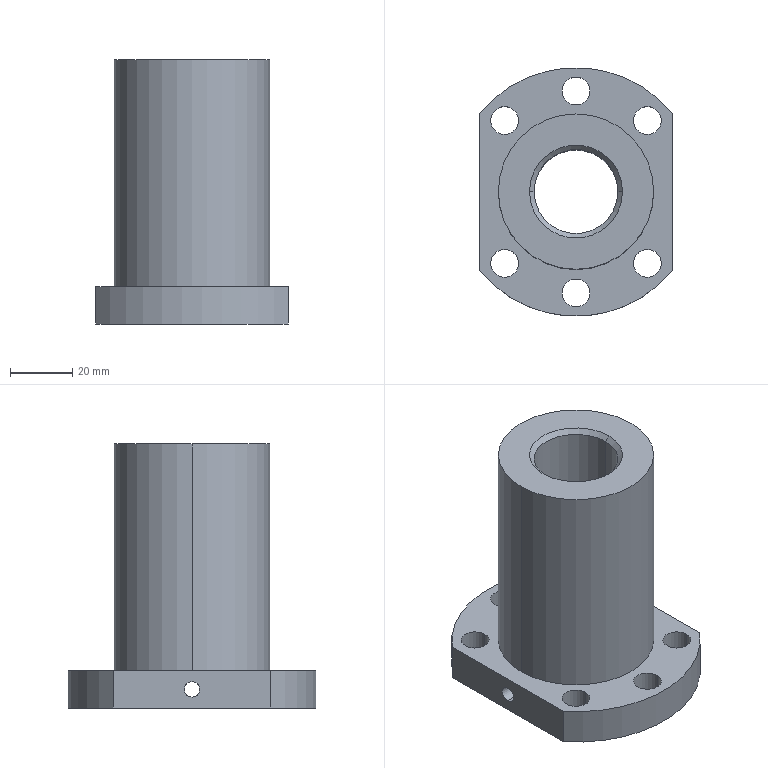Part | SolidWorks | features BaseBody 1 | 1 solid | 31 faces | box 62 x 80 x 85 mm | volume 142057 mm3 | cylinder 22 | plane 5 | cone 4 | commonest cylinder face diameters 9 x12 5 x4 27 x2 50 x2 80 x2
STEP:
#1=CARTESIAN_POINT('',(-25.,0.,85.));
#2=VERTEX_POINT('',#1);
#3=CARTESIAN_POINT('',(25.,0.,85.));
#4=VERTEX_POINT('',#3);
#5=CARTESIAN_POINT('',(0.,0.,85.));
#6=DIRECTION('',(0.,0.,-1.));
#7=DIRECTION('',(-1.,0.,0.));
#8=AXIS2_PLACEMENT_3D('',#5,#6,#7);
#9=CIRCLE('',#8,25.);
#10=EDGE_CURVE('',#2,#4,#9,.T.);
#11=ORIENTED_EDGE('',*,*,#10,.T.);
#12=CARTESIAN_POINT('',(25.,0.,12.));
#13=VERTEX_POINT('',#12);
#14=CARTESIAN_POINT('',(25.,0.,85.));
#15=DIRECTION('',(0.,0.,-1.));
#16=VECTOR('',#15,1000.);
#17=LINE('',#14,#16);
#18=EDGE_CURVE('',#4,#13,#17,.T.);
#19=ORIENTED_EDGE('',*,*,#18,.T.);
#20=CARTESIAN_POINT('',(-25.,0.,12.));
#21=VERTEX_POINT('',#20);
#22=CARTESIAN_POINT('',(0.,0.,12.));
#23=DIRECTION('',(0.,0.,1.));
#24=DIRECTION('',(-1.,0.,0.));
#25=AXIS2_PLACEMENT_3D('',#22,#23,#24);
#26=CIRCLE('',#25,25.);
#27=EDGE_CURVE('',#13,#21,#26,.T.);
#28=ORIENTED_EDGE('',*,*,#27,.T.);
#29=CARTESIAN_POINT('',(-25.,0.,85.));
#30=DIRECTION('',(0.,0.,-1.));
#31=VECTOR('',#30,1000.);
#32=LINE('',#29,#31);
#33=EDGE_CURVE('',#2,#21,#32,.T.);
#34=ORIENTED_EDGE('',*,*,#33,.F.);
#35=EDGE_LOOP('',(#11,#19,#28,#34));
#36=FACE_OUTER_BOUND('',#35,.T.);
#37=CARTESIAN_POINT('',(0.,0.,85.));
#38=DIRECTION('',(0.,0.,-1.));
#39=DIRECTION('',(-1.,0.,0.));
#40=AXIS2_PLACEMENT_3D('',#37,#38,#39);
#41=CYLINDRICAL_SURFACE('',#40,25.);
#42=ADVANCED_FACE('',(#36),#41,.T.);
#43=CARTESIAN_POINT('',(-18.481,-22.981,12.));
#44=VERTEX_POINT('',#43);
#45=CARTESIAN_POINT('',(-27.481,-22.981,12.));
#46=VERTEX_POINT('',#45);
#47=CARTESIAN_POINT('',(-22.981,-22.981,12.));
#48=DIRECTION('',(0.,0.,-1.));
#49=DIRECTION('',(-1.,0.,0.));
#50=AXIS2_PLACEMENT_3D('',#47,#48,#49);
#51=CIRCLE('',#50,4.5);
#52=EDGE_CURVE('',#44,#46,#51,.T.);
#53=ORIENTED_EDGE('',*,*,#52,.F.);
#54=CARTESIAN_POINT('',(-18.481,-22.981,0.));
#55=VERTEX_POINT('',#54);
#56=CARTESIAN_POINT('',(-18.481,-22.981,12.));
#57=DIRECTION('',(0.,0.,-1.));
#58=VECTOR('',#57,1000.);
#59=LINE('',#56,#58);
#60=EDGE_CURVE('',#44,#55,#59,.T.);
#61=ORIENTED_EDGE('',*,*,#60,.T.);
#62=CARTESIAN_POINT('',(-27.481,-22.981,0.));
#63=VERTEX_POINT('',#62);
#64=CARTESIAN_POINT('',(-22.981,-22.981,0.));
#65=DIRECTION('',(0.,0.,1.));
#66=DIRECTION('',(-1.,0.,0.));
#67=AXIS2_PLACEMENT_3D('',#64,#65,#66);
#68=CIRCLE('',#67,4.5);
#69=EDGE_CURVE('',#63,#55,#68,.T.);
#70=ORIENTED_EDGE('',*,*,#69,.F.);
#71=CARTESIAN_POINT('',(-27.481,-22.981,12.));
#72=DIRECTION('',(0.,0.,-1.));
#73=VECTOR('',#72,1000.);
#74=LINE('',#71,#73);
#75=EDGE_CURVE('',#46,#63,#74,.T.);
#76=ORIENTED_EDGE('',*,*,#75,.F.);
#77=EDGE_LOOP('',(#53,#61,#70,#76));
#78=FACE_OUTER_BOUND('',#77,.T.);
#79=CARTESIAN_POINT('',(-22.981,-22.981,12.));
#80=DIRECTION('',(0.,0.,-1.));
#81=DIRECTION('',(-1.,0.,0.));
#82=AXIS2_PLACEMENT_3D('',#79,#80,#81);
#83=CYLINDRICAL_SURFACE('',#82,4.5);
#84=ADVANCED_FACE('',(#78),#83,.F.);
#85=CARTESIAN_POINT('',(27.481,-22.981,12.));
#86=VERTEX_POINT('',#85);
#87=CARTESIAN_POINT('',(18.481,-22.981,12.));
#88=VERTEX_POINT('',#87);
#89=CARTESIAN_POINT('',(22.981,-22.981,12.));
#90=DIRECTION('',(0.,0.,-1.));
#91=DIRECTION('',(-1.,0.,0.));
#92=AXIS2_PLACEMENT_3D('',#89,#90,#91);
#93=CIRCLE('',#92,4.5);
#94=EDGE_CURVE('',#86,#88,#93,.T.);
#95=ORIENTED_EDGE('',*,*,#94,.F.);
#96=CARTESIAN_POINT('',(27.481,-22.981,0.));
#97=VERTEX_POINT('',#96);
#98=CARTESIAN_POINT('',(27.481,-22.981,12.));
#99=DIRECTION('',(0.,0.,-1.));
#100=VECTOR('',#99,1000.);
#101=LINE('',#98,#100);
#102=EDGE_CURVE('',#86,#97,#101,.T.);
#103=ORIENTED_EDGE('',*,*,#102,.T.);
#104=CARTESIAN_POINT('',(18.481,-22.981,0.));
#105=VERTEX_POINT('',#104);
#106=CARTESIAN_POINT('',(22.981,-22.981,0.));
#107=DIRECTION('',(0.,0.,1.));
#108=DIRECTION('',(-1.,0.,0.));
#109=AXIS2_PLACEMENT_3D('',#106,#107,#108);
#110=CIRCLE('',#109,4.5);
#111=EDGE_CURVE('',#105,#97,#110,.T.);
#112=ORIENTED_EDGE('',*,*,#111,.F.);
#113=CARTESIAN_POINT('',(18.481,-22.981,12.));
#114=DIRECTION('',(0.,0.,-1.));
#115=VECTOR('',#114,1000.);
#116=LINE('',#113,#115);
#117=EDGE_CURVE('',#88,#105,#116,.T.);
#118=ORIENTED_EDGE('',*,*,#117,.F.);
#119=EDGE_LOOP('',(#95,#103,#112,#118));
#120=FACE_OUTER_BOUND('',#119,.T.);
#121=CARTESIAN_POINT('',(22.981,-22.981,12.));
#122=DIRECTION('',(0.,0.,-1.));
#123=DIRECTION('',(-1.,0.,0.));
#124=AXIS2_PLACEMENT_3D('',#121,#122,#123);
#125=CYLINDRICAL_SURFACE('',#124,4.5);
#126=ADVANCED_FACE('',(#120),#125,.F.);
#127=CARTESIAN_POINT('',(27.481,22.981,12.));
#128=VERTEX_POINT('',#127);
#129=CARTESIAN_POINT('',(18.481,22.981,12.));
#130=VERTEX_POINT('',#129);
#131=CARTESIAN_POINT('',(22.981,22.981,12.));
#132=DIRECTION('',(0.,0.,-1.));
#133=DIRECTION('',(-1.,0.,0.));
#134=AXIS2_PLACEMENT_3D('',#131,#132,#133);
#135=CIRCLE('',#134,4.5);
#136=EDGE_CURVE('',#128,#130,#135,.T.);
#137=ORIENTED_EDGE('',*,*,#136,.F.);
#138=CARTESIAN_POINT('',(27.481,22.981,0.));
#139=VERTEX_POINT('',#138);
#140=CARTESIAN_POINT('',(27.481,22.981,12.));
#141=DIRECTION('',(0.,0.,-1.));
#142=VECTOR('',#141,1000.);
#143=LINE('',#140,#142);
#144=EDGE_CURVE('',#128,#139,#143,.T.);
#145=ORIENTED_EDGE('',*,*,#144,.T.);
#146=CARTESIAN_POINT('',(18.481,22.981,0.));
#147=VERTEX_POINT('',#146);
#148=CARTESIAN_POINT('',(22.981,22.981,0.));
#149=DIRECTION('',(0.,0.,1.));
#150=DIRECTION('',(-1.,0.,0.));
#151=AXIS2_PLACEMENT_3D('',#148,#149,#150);
#152=CIRCLE('',#151,4.5);
#153=EDGE_CURVE('',#147,#139,#152,.T.);
#154=ORIENTED_EDGE('',*,*,#153,.F.);
#155=CARTESIAN_POINT('',(18.481,22.981,12.));
#156=DIRECTION('',(0.,0.,-1.));
#157=VECTOR('',#156,1000.);
#158=LINE('',#155,#157);
#159=EDGE_CURVE('',#130,#147,#158,.T.);
#160=ORIENTED_EDGE('',*,*,#159,.F.);
#161=EDGE_LOOP('',(#137,#145,#154,#160));
#162=FACE_OUTER_BOUND('',#161,.T.);
#163=CARTESIAN_POINT('',(22.981,22.981,12.));
#164=DIRECTION('',(0.,0.,-1.));
#165=DIRECTION('',(-1.,0.,0.));
#166=AXIS2_PLACEMENT_3D('',#163,#164,#165);
#167=CYLINDRICAL_SURFACE('',#166,4.5);
#168=ADVANCED_FACE('',(#162),#167,.F.);
#169=CARTESIAN_POINT('',(4.5,32.5,12.));
#170=VERTEX_POINT('',#169);
#171=CARTESIAN_POINT('',(-4.5,32.5,12.));
#172=VERTEX_POINT('',#171);
#173=CARTESIAN_POINT('',(0.,32.5,12.));
#174=DIRECTION('',(0.,0.,-1.));
#175=DIRECTION('',(-1.,0.,0.));
#176=AXIS2_PLACEMENT_3D('',#173,#174,#175);
#177=CIRCLE('',#176,4.5);
#178=EDGE_CURVE('',#170,#172,#177,.T.);
#179=ORIENTED_EDGE('',*,*,#178,.F.);
#180=CARTESIAN_POINT('',(4.5,32.5,0.));
#181=VERTEX_POINT('',#180);
#182=CARTESIAN_POINT('',(4.5,32.5,12.));
#183=DIRECTION('',(0.,0.,-1.));
#184=VECTOR('',#183,1000.);
#185=LINE('',#182,#184);
#186=EDGE_CURVE('',#170,#181,#185,.T.);
#187=ORIENTED_EDGE('',*,*,#186,.T.);
#188=CARTESIAN_POINT('',(-4.5,32.5,0.));
#189=VERTEX_POINT('',#188);
#190=CARTESIAN_POINT('',(0.,32.5,0.));
#191=DIRECTION('',(0.,0.,1.));
#192=DIRECTION('',(-1.,0.,0.));
#193=AXIS2_PLACEMENT_3D('',#190,#191,#192);
#194=CIRCLE('',#193,4.5);
#195=EDGE_CURVE('',#189,#181,#194,.T.);
#196=ORIENTED_EDGE('',*,*,#195,.F.);
#197=CARTESIAN_POINT('',(-4.5,32.5,12.));
#198=DIRECTION('',(0.,0.,-1.));
#199=VECTOR('',#198,1000.);
#200=LINE('',#197,#199);
#201=EDGE_CURVE('',#172,#189,#200,.T.);
#202=ORIENTED_EDGE('',*,*,#201,.F.);
#203=EDGE_LOOP('',(#179,#187,#196,#202));
#204=FACE_OUTER_BOUND('',#203,.T.);
#205=CARTESIAN_POINT('',(0.,32.5,12.));
#206=DIRECTION('',(0.,0.,-1.));
#207=DIRECTION('',(-1.,0.,0.));
#208=AXIS2_PLACEMENT_3D('',#205,#206,#207);
#209=CYLINDRICAL_SURFACE('',#208,4.5);
#210=ADVANCED_FACE('',(#204),#209,.F.);
#211=CARTESIAN_POINT('',(-18.481,22.981,12.));
#212=VERTEX_POINT('',#211);
#213=CARTESIAN_POINT('',(-27.481,22.981,12.));
#214=VERTEX_POINT('',#213);
#215=CARTESIAN_POINT('',(-22.981,22.981,12.));
#216=DIRECTION('',(0.,0.,-1.));
#217=DIRECTION('',(-1.,0.,0.));
#218=AXIS2_PLACEMENT_3D('',#215,#216,#217);
#219=CIRCLE('',#218,4.5);
#220=EDGE_CURVE('',#212,#214,#219,.T.);
#221=ORIENTED_EDGE('',*,*,#220,.F.);
#222=CARTESIAN_POINT('',(-18.481,22.981,0.));
#223=VERTEX_POINT('',#222);
#224=CARTESIAN_POINT('',(-18.481,22.981,12.));
#225=DIRECTION('',(0.,0.,-1.));
#226=VECTOR('',#225,1000.);
#227=LINE('',#224,#226);
#228=EDGE_CURVE('',#212,#223,#227,.T.);
#229=ORIENTED_EDGE('',*,*,#228,.T.);
#230=CARTESIAN_POINT('',(-27.481,22.981,0.));
#231=VERTEX_POINT('',#230);
#232=CARTESIAN_POINT('',(-22.981,22.981,0.));
#233=DIRECTION('',(0.,0.,1.));
#234=DIRECTION('',(-1.,0.,0.));
#235=AXIS2_PLACEMENT_3D('',#232,#233,#234);
#236=CIRCLE('',#235,4.5);
#237=EDGE_CURVE('',#231,#223,#236,.T.);
#238=ORIENTED_EDGE('',*,*,#237,.F.);
#239=CARTESIAN_POINT('',(-27.481,22.981,12.));
#240=DIRECTION('',(0.,0.,-1.));
#241=VECTOR('',#240,1000.);
#242=LINE('',#239,#241);
#243=EDGE_CURVE('',#214,#231,#242,.T.);
#244=ORIENTED_EDGE('',*,*,#243,.F.);
#245=EDGE_LOOP('',(#221,#229,#238,#244));
#246=FACE_OUTER_BOUND('',#245,.T.);
#247=CARTESIAN_POINT('',(-22.981,22.981,12.));
#248=DIRECTION('',(0.,0.,-1.));
#249=DIRECTION('',(-1.,0.,0.));
#250=AXIS2_PLACEMENT_3D('',#247,#248,#249);
#251=CYLINDRICAL_SURFACE('',#250,4.5);
#252=ADVANCED_FACE('',(#246),#251,.F.);
#253=CARTESIAN_POINT('',(4.5,-32.5,12.));
#254=VERTEX_POINT('',#253);
#255=CARTESIAN_POINT('',(-4.5,-32.5,12.));
#256=VERTEX_POINT('',#255);
#257=CARTESIAN_POINT('',(0.,-32.5,12.));
#258=DIRECTION('',(0.,0.,-1.));
#259=DIRECTION('',(-1.,0.,0.));
#260=AXIS2_PLACEMENT_3D('',#257,#258,#259);
#261=CIRCLE('',#260,4.5);
#262=EDGE_CURVE('',#254,#256,#261,.T.);
#263=ORIENTED_EDGE('',*,*,#262,.F.);
#264=CARTESIAN_POINT('',(4.5,-32.5,0.));
#265=VERTEX_POINT('',#264);
#266=CARTESIAN_POINT('',(4.5,-32.5,12.));
#267=DIRECTION('',(0.,0.,-1.));
#268=VECTOR('',#267,1000.);
#269=LINE('',#266,#268);
#270=EDGE_CURVE('',#254,#265,#269,.T.);
#271=ORIENTED_EDGE('',*,*,#270,.T.);
#272=CARTESIAN_POINT('',(-4.5,-32.5,0.));
#273=VERTEX_POINT('',#272);
#274=CARTESIAN_POINT('',(0.,-32.5,0.));
#275=DIRECTION('',(0.,0.,1.));
#276=DIRECTION('',(-1.,0.,0.));
#277=AXIS2_PLACEMENT_3D('',#274,#275,#276);
#278=CIRCLE('',#277,4.5);
#279=EDGE_CURVE('',#273,#265,#278,.T.);
#280=ORIENTED_EDGE('',*,*,#279,.F.);
#281=CARTESIAN_POINT('',(-4.5,-32.5,12.));
#282=DIRECTION('',(0.,0.,-1.));
#283=VECTOR('',#282,1000.);
#284=LINE('',#281,#283);
#285=EDGE_CURVE('',#256,#273,#284,.T.);
#286=ORIENTED_EDGE('',*,*,#285,.F.);
#287=EDGE_LOOP('',(#263,#271,#280,#286));
#288=FACE_OUTER_BOUND('',#287,.T.);
#289=CARTESIAN_POINT('',(0.,-32.5,12.));
#290=DIRECTION('',(0.,0.,-1.));
#291=DIRECTION('',(-1.,0.,0.));
#292=AXIS2_PLACEMENT_3D('',#289,#290,#291);
#293=CYLINDRICAL_SURFACE('',#292,4.5);
#294=ADVANCED_FACE('',(#288),#293,.F.);
#295=CARTESIAN_POINT('',(-13.5,0.,83.5));
#296=VERTEX_POINT('',#295);
#297=CARTESIAN_POINT('',(13.5,0.,83.5));
#298=VERTEX_POINT('',#297);
#299=CARTESIAN_POINT('',(0.,0.,83.5));
#300=DIRECTION('',(0.,0.,1.));
#301=DIRECTION('',(1.,0.,0.));
#302=AXIS2_PLACEMENT_3D('',#299,#300,#301);
#303=CIRCLE('',#302,13.5);
#304=EDGE_CURVE('',#296,#298,#303,.T.);
#305=ORIENTED_EDGE('',*,*,#304,.F.);
#306=CARTESIAN_POINT('',(-15.,0.,85.));
#307=VERTEX_POINT('',#306);
#308=CARTESIAN_POINT('',(-15.,0.,85.));
#309=DIRECTION('',(-0.7071,0.,0.7071));
#310=VECTOR('',#309,1000.);
#311=LINE('',#308,#310);
#312=EDGE_CURVE('',#296,#307,#311,.T.);
#313=ORIENTED_EDGE('',*,*,#312,.T.);
#314=CARTESIAN_POINT('',(15.,0.,85.));
#315=VERTEX_POINT('',#314);
#316=CARTESIAN_POINT('',(0.,0.,85.));
#317=DIRECTION('',(0.,0.,-1.));
#318=DIRECTION('',(1.,0.,0.));
#319=AXIS2_PLACEMENT_3D('',#316,#317,#318);
#320=CIRCLE('',#319,15.);
#321=EDGE_CURVE('',#315,#307,#320,.T.);
#322=ORIENTED_EDGE('',*,*,#321,.F.);
#323=CARTESIAN_POINT('',(15.,0.,85.));
#324=DIRECTION('',(0.7071,0.,0.7071));
#325=VECTOR('',#324,1000.);
#326=LINE('',#323,#325);
#327=EDGE_CURVE('',#298,#315,#326,.T.);
#328=ORIENTED_EDGE('',*,*,#327,.F.);
#329=EDGE_LOOP('',(#305,#313,#322,#328));
#330=FACE_OUTER_BOUND('',#329,.T.);
#331=CARTESIAN_POINT('',(0.,0.,85.));
#332=DIRECTION('',(0.,0.,1.));
#333=DIRECTION('',(1.,0.,0.));
#334=AXIS2_PLACEMENT_3D('',#331,#332,#333);
#335=CONICAL_SURFACE('',#334,15.,0.7854);
#336=ADVANCED_FACE('',(#330),#335,.F.);
#337=CARTESIAN_POINT('',(-13.5,0.,3.5));
#338=VERTEX_POINT('',#337);
#339=CARTESIAN_POINT('',(-13.5,0.,8.5));
#340=VERTEX_POINT('',#339);
#341=CARTESIAN_POINT('',(-13.5,0.,3.5));
#342=CARTESIAN_POINT('',(-13.5,-0.1655,3.5));
#343=CARTESIAN_POINT('',(-13.497,-0.3282,3.516));
#344=CARTESIAN_POINT('',(-13.485,-0.6482,3.58));
#345=CARTESIAN_POINT('',(-13.477,-0.8071,3.628));
#346=CARTESIAN_POINT('',(-13.455,-1.11,3.754));
#347=CARTESIAN_POINT('',(-13.442,-1.253,3.831));
#348=CARTESIAN_POINT('',(-13.414,-1.525,4.012));
#349=CARTESIAN_POINT('',(-13.399,-1.653,4.117));
#350=CARTESIAN_POINT('',(-13.353,-1.998,4.462));
#351=CARTESIAN_POINT('',(-13.323,-2.184,4.741));
#352=CARTESIAN_POINT('',(-13.29,-2.371,5.191));
#353=CARTESIAN_POINT('',(-13.281,-2.419,5.349));
#354=CARTESIAN_POINT('',(-13.27,-2.484,5.672));
#355=CARTESIAN_POINT('',(-13.267,-2.5,5.835));
#356=CARTESIAN_POINT('',(-13.266,-2.5,6.161));
#357=CARTESIAN_POINT('',(-13.27,-2.484,6.327));
#358=CARTESIAN_POINT('',(-13.281,-2.42,6.648));
#359=CARTESIAN_POINT('',(-13.29,-2.373,6.804));
#360=CARTESIAN_POINT('',(-13.312,-2.247,7.107));
#361=CARTESIAN_POINT('',(-13.325,-2.169,7.253));
#362=CARTESIAN_POINT('',(-13.353,-1.989,7.524));
#363=CARTESIAN_POINT('',(-13.368,-1.885,7.65));
#364=CARTESIAN_POINT('',(-13.399,-1.653,7.883));
#365=CARTESIAN_POINT('',(-13.414,-1.527,7.986));
#366=CARTESIAN_POINT('',(-13.442,-1.257,8.167));
#367=CARTESIAN_POINT('',(-13.455,-1.11,8.246));
#368=CARTESIAN_POINT('',(-13.477,-0.8081,8.371));
#369=CARTESIAN_POINT('',(-13.485,-0.6523,8.419));
#370=CARTESIAN_POINT('',(-13.497,-0.3312,8.483));
#371=CARTESIAN_POINT('',(-13.5,-0.1655,8.5));
#372=CARTESIAN_POINT('',(-13.5,0.,8.5));
#373=B_SPLINE_CURVE_WITH_KNOTS('',3,(#341,#342,#343,#344,#345,#346,#347,#348,#349,#350,#351,#352,#353,#354,#355,#356,#357,#358,#359,#360,#361,#362,#363,#364,#365,#366,#367,#368,#369,#370,#371,#372),.UNSPECIFIED.,.F.,.F.,(4,2,2,2,2,2,2,2,2,2,2,2,2,2,2,4),(0.,0.0004894,0.0009789,0.001468,0.001958,0.002937,0.003426,0.003916,0.004405,0.004894,0.005384,0.005873,0.006363,0.006852,0.007342,0.007831),.UNSPECIFIED.);
#374=EDGE_CURVE('',#338,#340,#373,.T.);
#375=ORIENTED_EDGE('',*,*,#374,.F.);
#376=CARTESIAN_POINT('',(-31.,0.,3.5));
#377=VERTEX_POINT('',#376);
#378=CARTESIAN_POINT('',(-31.,0.,3.5));
#379=DIRECTION('',(-1.,0.,0.));
#380=VECTOR('',#379,1000.);
#381=LINE('',#378,#380);
#382=EDGE_CURVE('',#338,#377,#381,.T.);
#383=ORIENTED_EDGE('',*,*,#382,.T.);
#384=CARTESIAN_POINT('',(-31.,0.,8.5));
#385=VERTEX_POINT('',#384);
#386=CARTESIAN_POINT('',(-31.,0.,6.));
#387=DIRECTION('',(1.,0.,0.));
#388=DIRECTION('',(0.,0.,1.));
#389=AXIS2_PLACEMENT_3D('',#386,#387,#388);
#390=CIRCLE('',#389,2.5);
#391=EDGE_CURVE('',#385,#377,#390,.T.);
#392=ORIENTED_EDGE('',*,*,#391,.F.);
#393=CARTESIAN_POINT('',(-31.,0.,8.5));
#394=DIRECTION('',(-1.,0.,0.));
#395=VECTOR('',#394,1000.);
#396=LINE('',#393,#395);
#397=EDGE_CURVE('',#340,#385,#396,.T.);
#398=ORIENTED_EDGE('',*,*,#397,.F.);
#399=EDGE_LOOP('',(#375,#383,#392,#398));
#400=FACE_OUTER_BOUND('',#399,.T.);
#401=CARTESIAN_POINT('',(-31.,0.,6.));
#402=DIRECTION('',(-1.,0.,0.));
#403=DIRECTION('',(0.,0.,1.));
#404=AXIS2_PLACEMENT_3D('',#401,#402,#403);
#405=CYLINDRICAL_SURFACE('',#404,2.5);
#406=ADVANCED_FACE('',(#400),#405,.F.);
#407=CARTESIAN_POINT('',(31.,0.,3.5));
#408=VERTEX_POINT('',#407);
#409=CARTESIAN_POINT('',(31.,0.,8.5));
#410=VERTEX_POINT('',#409);
#411=CARTESIAN_POINT('',(31.,0.,6.));
#412=DIRECTION('',(-1.,0.,0.));
#413=DIRECTION('',(0.,0.,1.));
#414=AXIS2_PLACEMENT_3D('',#411,#412,#413);
#415=CIRCLE('',#414,2.5);
#416=EDGE_CURVE('',#408,#410,#415,.T.);
#417=ORIENTED_EDGE('',*,*,#416,.F.);
#418=CARTESIAN_POINT('',(13.5,0.,3.5));
#419=VERTEX_POINT('',#418);
#420=CARTESIAN_POINT('',(-31.,0.,3.5));
#421=DIRECTION('',(-1.,0.,0.));
#422=VECTOR('',#421,1000.);
#423=LINE('',#420,#422);
#424=EDGE_CURVE('',#408,#419,#423,.T.);
#425=ORIENTED_EDGE('',*,*,#424,.T.);
#426=CARTESIAN_POINT('',(13.5,0.,8.5));
#427=VERTEX_POINT('',#426);
#428=CARTESIAN_POINT('',(13.5,0.,8.5));
#429=CARTESIAN_POINT('',(13.5,-0.1655,8.5));
#430=CARTESIAN_POINT('',(13.497,-0.3282,8.484));
#431=CARTESIAN_POINT('',(13.485,-0.6482,8.42));
#432=CARTESIAN_POINT('',(13.477,-0.8071,8.372));
#433=CARTESIAN_POINT('',(13.455,-1.11,8.246));
#434=CARTESIAN_POINT('',(13.442,-1.253,8.169));
#435=CARTESIAN_POINT('',(13.414,-1.525,7.988));
#436=CARTESIAN_POINT('',(13.399,-1.653,7.883));
#437=CARTESIAN_POINT('',(13.353,-1.998,7.538));
#438=CARTESIAN_POINT('',(13.323,-2.184,7.259));
#439=CARTESIAN_POINT('',(13.29,-2.371,6.809));
#440=CARTESIAN_POINT('',(13.281,-2.419,6.651));
#441=CARTESIAN_POINT('',(13.27,-2.484,6.328));
#442=CARTESIAN_POINT('',(13.267,-2.5,6.165));
#443=CARTESIAN_POINT('',(13.266,-2.5,5.839));
#444=CARTESIAN_POINT('',(13.27,-2.484,5.673));
#445=CARTESIAN_POINT('',(13.281,-2.42,5.352));
#446=CARTESIAN_POINT('',(13.29,-2.373,5.196));
#447=CARTESIAN_POINT('',(13.312,-2.247,4.893));
#448=CARTESIAN_POINT('',(13.325,-2.169,4.747));
#449=CARTESIAN_POINT('',(13.353,-1.989,4.476));
#450=CARTESIAN_POINT('',(13.368,-1.885,4.35));
#451=CARTESIAN_POINT('',(13.399,-1.653,4.117));
#452=CARTESIAN_POINT('',(13.414,-1.527,4.014));
#453=CARTESIAN_POINT('',(13.442,-1.257,3.833));
#454=CARTESIAN_POINT('',(13.455,-1.11,3.754));
#455=CARTESIAN_POINT('',(13.477,-0.8081,3.629));
#456=CARTESIAN_POINT('',(13.485,-0.6523,3.581));
#457=CARTESIAN_POINT('',(13.497,-0.3312,3.517));
#458=CARTESIAN_POINT('',(13.5,-0.1655,3.5));
#459=CARTESIAN_POINT('',(13.5,0.,3.5));
#460=B_SPLINE_CURVE_WITH_KNOTS('',3,(#428,#429,#430,#431,#432,#433,#434,#435,#436,#437,#438,#439,#440,#441,#442,#443,#444,#445,#446,#447,#448,#449,#450,#451,#452,#453,#454,#455,#456,#457,#458,#459),.UNSPECIFIED.,.F.,.F.,(4,2,2,2,2,2,2,2,2,2,2,2,2,2,2,4),(0.,0.0004894,0.0009789,0.001468,0.001958,0.002937,0.003426,0.003916,0.004405,0.004894,0.005384,0.005873,0.006363,0.006852,0.007342,0.007831),.UNSPECIFIED.);
#461=EDGE_CURVE('',#427,#419,#460,.T.);
#462=ORIENTED_EDGE('',*,*,#461,.F.);
#463=CARTESIAN_POINT('',(-31.,0.,8.5));
#464=DIRECTION('',(-1.,0.,0.));
#465=VECTOR('',#464,1000.);
#466=LINE('',#463,#465);
#467=EDGE_CURVE('',#410,#427,#466,.T.);
#468=ORIENTED_EDGE('',*,*,#467,.F.);
#469=EDGE_LOOP('',(#417,#425,#462,#468));
#470=FACE_OUTER_BOUND('',#469,.T.);
#471=CARTESIAN_POINT('',(-31.,0.,6.));
#472=DIRECTION('',(-1.,0.,0.));
#473=DIRECTION('',(0.,0.,1.));
#474=AXIS2_PLACEMENT_3D('',#471,#472,#473);
#475=CYLINDRICAL_SURFACE('',#474,2.5);
#476=ADVANCED_FACE('',(#470),#475,.F.);
#477=ORIENTED_EDGE('',*,*,#304,.T.);
#478=CARTESIAN_POINT('',(13.5,0.,85.));
#479=DIRECTION('',(0.,0.,-1.));
#480=VECTOR('',#479,1000.);
#481=LINE('',#478,#480);
#482=EDGE_CURVE('',#298,#427,#481,.T.);
#483=ORIENTED_EDGE('',*,*,#482,.T.);
#484=ORIENTED_EDGE('',*,*,#461,.T.);
#485=CARTESIAN_POINT('',(13.5,0.,1.5));
#486=VERTEX_POINT('',#485);
#487=CARTESIAN_POINT('',(13.5,0.,85.));
#488=DIRECTION('',(0.,0.,-1.));
#489=VECTOR('',#488,1000.);
#490=LINE('',#487,#489);
#491=EDGE_CURVE('',#419,#486,#490,.T.);
#492=ORIENTED_EDGE('',*,*,#491,.T.);
#493=CARTESIAN_POINT('',(-13.5,0.,1.5));
#494=VERTEX_POINT('',#493);
#495=CARTESIAN_POINT('',(0.,0.,1.5));
#496=DIRECTION('',(0.,0.,1.));
#497=DIRECTION('',(-1.,0.,0.));
#498=AXIS2_PLACEMENT_3D('',#495,#496,#497);
#499=CIRCLE('',#498,13.5);
#500=EDGE_CURVE('',#494,#486,#499,.T.);
#501=ORIENTED_EDGE('',*,*,#500,.F.);
#502=CARTESIAN_POINT('',(-13.5,0.,85.));
#503=DIRECTION('',(0.,0.,-1.));
#504=VECTOR('',#503,1000.);
#505=LINE('',#502,#504);
#506=EDGE_CURVE('',#338,#494,#505,.T.);
#507=ORIENTED_EDGE('',*,*,#506,.F.);
#508=ORIENTED_EDGE('',*,*,#374,.T.);
#509=CARTESIAN_POINT('',(-13.5,0.,85.));
#510=DIRECTION('',(0.,0.,-1.));
#511=VECTOR('',#510,1000.);
#512=LINE('',#509,#511);
#513=EDGE_CURVE('',#296,#340,#512,.T.);
#514=ORIENTED_EDGE('',*,*,#513,.F.);
#515=EDGE_LOOP('',(#477,#483,#484,#492,#501,#507,#508,#514));
#516=FACE_OUTER_BOUND('',#515,.T.);
#517=CARTESIAN_POINT('',(0.,0.,85.));
#518=DIRECTION('',(0.,0.,-1.));
#519=DIRECTION('',(-1.,0.,0.));
#520=AXIS2_PLACEMENT_3D('',#517,#518,#519);
#521=CYLINDRICAL_SURFACE('',#520,13.5);
#522=ADVANCED_FACE('',(#516),#521,.F.);
#523=ORIENTED_EDGE('',*,*,#500,.T.);
#524=CARTESIAN_POINT('',(15.,0.,0.));
#525=VERTEX_POINT('',#524);
#526=CARTESIAN_POINT('',(15.,0.,0.));
#527=DIRECTION('',(0.7071,0.,-0.7071));
#528=VECTOR('',#527,1000.);
#529=LINE('',#526,#528);
#530=EDGE_CURVE('',#486,#525,#529,.T.);
#531=ORIENTED_EDGE('',*,*,#530,.T.);
#532=CARTESIAN_POINT('',(-15.,0.,0.));
#533=VERTEX_POINT('',#532);
#534=CARTESIAN_POINT('',(0.,0.,0.));
#535=DIRECTION('',(0.,0.,-1.));
#536=DIRECTION('',(-1.,0.,0.));
#537=AXIS2_PLACEMENT_3D('',#534,#535,#536);
#538=CIRCLE('',#537,15.);
#539=EDGE_CURVE('',#525,#533,#538,.T.);
#540=ORIENTED_EDGE('',*,*,#539,.T.);
#541=CARTESIAN_POINT('',(-15.,0.,0.));
#542=DIRECTION('',(-0.7071,0.,-0.7071));
#543=VECTOR('',#542,1000.);
#544=LINE('',#541,#543);
#545=EDGE_CURVE('',#494,#533,#544,.T.);
#546=ORIENTED_EDGE('',*,*,#545,.F.);
#547=EDGE_LOOP('',(#523,#531,#540,#546));
#548=FACE_OUTER_BOUND('',#547,.T.);
#549=CARTESIAN_POINT('',(0.,0.,0.));
#550=DIRECTION('',(0.,0.,-1.));
#551=DIRECTION('',(-1.,0.,0.));
#552=AXIS2_PLACEMENT_3D('',#549,#550,#551);
#553=CONICAL_SURFACE('',#552,15.,0.7854);
#554=ADVANCED_FACE('',(#548),#553,.F.);
#555=ORIENTED_EDGE('',*,*,#18,.F.);
#556=CARTESIAN_POINT('',(0.,0.,85.));
#557=DIRECTION('',(0.,0.,-1.));
#558=DIRECTION('',(-1.,0.,0.));
#559=AXIS2_PLACEMENT_3D('',#556,#557,#558);
#560=CIRCLE('',#559,25.);
#561=EDGE_CURVE('',#4,#2,#560,.T.);
#562=ORIENTED_EDGE('',*,*,#561,.T.);
#563=ORIENTED_EDGE('',*,*,#33,.T.);
#564=CARTESIAN_POINT('',(0.,0.,12.));
#565=DIRECTION('',(0.,0.,1.));
#566=DIRECTION('',(-1.,0.,0.));
#567=AXIS2_PLACEMENT_3D('',#564,#565,#566);
#568=CIRCLE('',#567,25.);
#569=EDGE_CURVE('',#21,#13,#568,.T.);
#570=ORIENTED_EDGE('',*,*,#569,.T.);
#571=EDGE_LOOP('',(#555,#562,#563,#570));
#572=FACE_OUTER_BOUND('',#571,.T.);
#573=CARTESIAN_POINT('',(0.,0.,85.));
#574=DIRECTION('',(0.,0.,-1.));
#575=DIRECTION('',(-1.,0.,0.));
#576=AXIS2_PLACEMENT_3D('',#573,#574,#575);
#577=CYLINDRICAL_SURFACE('',#576,25.);
#578=ADVANCED_FACE('',(#572),#577,.T.);
#579=CARTESIAN_POINT('',(-22.981,-22.981,12.));
#580=DIRECTION('',(0.,0.,-1.));
#581=DIRECTION('',(-1.,0.,0.));
#582=AXIS2_PLACEMENT_3D('',#579,#580,#581);
#583=CIRCLE('',#582,4.5);
#584=EDGE_CURVE('',#46,#44,#583,.T.);
#585=ORIENTED_EDGE('',*,*,#584,.T.);
#586=ORIENTED_EDGE('',*,*,#52,.T.);
#587=EDGE_LOOP('',(#585,#586));
#588=FACE_BOUND('',#587,.T.);
#589=CARTESIAN_POINT('',(22.981,-22.981,12.));
#590=DIRECTION('',(0.,0.,-1.));
#591=DIRECTION('',(-1.,0.,0.));
#592=AXIS2_PLACEMENT_3D('',#589,#590,#591);
#593=CIRCLE('',#592,4.5);
#594=EDGE_CURVE('',#88,#86,#593,.T.);
#595=ORIENTED_EDGE('',*,*,#594,.T.);
#596=ORIENTED_EDGE('',*,*,#94,.T.);
#597=EDGE_LOOP('',(#595,#596));
#598=FACE_BOUND('',#597,.T.);
#599=CARTESIAN_POINT('',(22.981,22.981,12.));
#600=DIRECTION('',(0.,0.,-1.));
#601=DIRECTION('',(-1.,0.,0.));
#602=AXIS2_PLACEMENT_3D('',#599,#600,#601);
#603=CIRCLE('',#602,4.5);
#604=EDGE_CURVE('',#130,#128,#603,.T.);
#605=ORIENTED_EDGE('',*,*,#604,.T.);
#606=ORIENTED_EDGE('',*,*,#136,.T.);
#607=EDGE_LOOP('',(#605,#606));
#608=FACE_BOUND('',#607,.T.);
#609=CARTESIAN_POINT('',(0.,32.5,12.));
#610=DIRECTION('',(0.,0.,-1.));
#611=DIRECTION('',(-1.,0.,0.));
#612=AXIS2_PLACEMENT_3D('',#609,#610,#611);
#613=CIRCLE('',#612,4.5);
#614=EDGE_CURVE('',#172,#170,#613,.T.);
#615=ORIENTED_EDGE('',*,*,#614,.T.);
#616=ORIENTED_EDGE('',*,*,#178,.T.);
#617=EDGE_LOOP('',(#615,#616));
#618=FACE_BOUND('',#617,.T.);
#619=CARTESIAN_POINT('',(-22.981,22.981,12.));
#620=DIRECTION('',(0.,0.,-1.));
#621=DIRECTION('',(-1.,0.,0.));
#622=AXIS2_PLACEMENT_3D('',#619,#620,#621);
#623=CIRCLE('',#622,4.5);
#624=EDGE_CURVE('',#214,#212,#623,.T.);
#625=ORIENTED_EDGE('',*,*,#624,.T.);
#626=ORIENTED_EDGE('',*,*,#220,.T.);
#627=EDGE_LOOP('',(#625,#626));
#628=FACE_BOUND('',#627,.T.);
#629=CARTESIAN_POINT('',(0.,-32.5,12.));
#630=DIRECTION('',(0.,0.,-1.));
#631=DIRECTION('',(-1.,0.,0.));
#632=AXIS2_PLACEMENT_3D('',#629,#630,#631);
#633=CIRCLE('',#632,4.5);
#634=EDGE_CURVE('',#256,#254,#633,.T.);
#635=ORIENTED_EDGE('',*,*,#634,.T.);
#636=ORIENTED_EDGE('',*,*,#262,.T.);
#637=EDGE_LOOP('',(#635,#636));
#638=FACE_BOUND('',#637,.T.);
#639=ORIENTED_EDGE('',*,*,#569,.F.);
#640=ORIENTED_EDGE('',*,*,#27,.F.);
#641=EDGE_LOOP('',(#639,#640));
#642=FACE_BOUND('',#641,.T.);
#643=CARTESIAN_POINT('',(31.,25.278,12.));
#644=VERTEX_POINT('',#643);
#645=CARTESIAN_POINT('',(-31.,25.278,12.));
#646=VERTEX_POINT('',#645);
#647=CARTESIAN_POINT('',(0.,0.,12.));
#648=DIRECTION('',(0.,0.,1.));
#649=DIRECTION('',(-1.,0.,0.));
#650=AXIS2_PLACEMENT_3D('',#647,#648,#649);
#651=CIRCLE('',#650,40.);
#652=EDGE_CURVE('',#644,#646,#651,.T.);
#653=ORIENTED_EDGE('',*,*,#652,.T.);
#654=CARTESIAN_POINT('',(-31.,-25.278,12.));
#655=VERTEX_POINT('',#654);
#656=CARTESIAN_POINT('',(-31.,0.,12.));
#657=DIRECTION('',(0.,-1.,0.));
#658=VECTOR('',#657,1000.);
#659=LINE('',#656,#658);
#660=EDGE_CURVE('',#646,#655,#659,.T.);
#661=ORIENTED_EDGE('',*,*,#660,.T.);
#662=CARTESIAN_POINT('',(31.,-25.278,12.));
#663=VERTEX_POINT('',#662);
#664=CARTESIAN_POINT('',(0.,0.,12.));
#665=DIRECTION('',(0.,0.,1.));
#666=DIRECTION('',(-1.,0.,0.));
#667=AXIS2_PLACEMENT_3D('',#664,#665,#666);
#668=CIRCLE('',#667,40.);
#669=EDGE_CURVE('',#655,#663,#668,.T.);
#670=ORIENTED_EDGE('',*,*,#669,.T.);
#671=CARTESIAN_POINT('',(31.,0.,12.));
#672=DIRECTION('',(0.,1.,0.));
#673=VECTOR('',#672,1000.);
#674=LINE('',#671,#673);
#675=EDGE_CURVE('',#663,#644,#674,.T.);
#676=ORIENTED_EDGE('',*,*,#675,.T.);
#677=EDGE_LOOP('',(#653,#661,#670,#676));
#678=FACE_OUTER_BOUND('',#677,.T.);
#679=CARTESIAN_POINT('',(0.,0.,12.));
#680=DIRECTION('',(0.,0.,1.));
#681=DIRECTION('',(1.,0.,0.));
#682=AXIS2_PLACEMENT_3D('',#679,#680,#681);
#683=PLANE('',#682);
#684=ADVANCED_FACE('',(#588,#598,#608,#618,#628,#638,#642,#678),#683,.T.);
#685=ORIENTED_EDGE('',*,*,#321,.T.);
#686=CARTESIAN_POINT('',(0.,0.,85.));
#687=DIRECTION('',(0.,0.,-1.));
#688=DIRECTION('',(1.,0.,0.));
#689=AXIS2_PLACEMENT_3D('',#686,#687,#688);
#690=CIRCLE('',#689,15.);
#691=EDGE_CURVE('',#307,#315,#690,.T.);
#692=ORIENTED_EDGE('',*,*,#691,.T.);
#693=EDGE_LOOP('',(#685,#692));
#694=FACE_BOUND('',#693,.T.);
#695=ORIENTED_EDGE('',*,*,#10,.F.);
#696=ORIENTED_EDGE('',*,*,#561,.F.);
#697=EDGE_LOOP('',(#695,#696));
#698=FACE_OUTER_BOUND('',#697,.T.);
#699=CARTESIAN_POINT('',(0.,0.,85.));
#700=DIRECTION('',(0.,0.,1.));
#701=DIRECTION('',(1.,0.,0.));
#702=AXIS2_PLACEMENT_3D('',#699,#700,#701);
#703=PLANE('',#702);
#704=ADVANCED_FACE('',(#694,#698),#703,.T.);
#705=ORIENTED_EDGE('',*,*,#60,.F.);
#706=ORIENTED_EDGE('',*,*,#584,.F.);
#707=ORIENTED_EDGE('',*,*,#75,.T.);
#708=CARTESIAN_POINT('',(-22.981,-22.981,0.));
#709=DIRECTION('',(0.,0.,1.));
#710=DIRECTION('',(-1.,0.,0.));
#711=AXIS2_PLACEMENT_3D('',#708,#709,#710);
#712=CIRCLE('',#711,4.5);
#713=EDGE_CURVE('',#55,#63,#712,.T.);
#714=ORIENTED_EDGE('',*,*,#713,.F.);
#715=EDGE_LOOP('',(#705,#706,#707,#714));
#716=FACE_OUTER_BOUND('',#715,.T.);
#717=CARTESIAN_POINT('',(-22.981,-22.981,12.));
#718=DIRECTION('',(0.,0.,-1.));
#719=DIRECTION('',(-1.,0.,0.));
#720=AXIS2_PLACEMENT_3D('',#717,#718,#719);
#721=CYLINDRICAL_SURFACE('',#720,4.5);
#722=ADVANCED_FACE('',(#716),#721,.F.);
#723=ORIENTED_EDGE('',*,*,#102,.F.);
#724=ORIENTED_EDGE('',*,*,#594,.F.);
#725=ORIENTED_EDGE('',*,*,#117,.T.);
#726=CARTESIAN_POINT('',(22.981,-22.981,0.));
#727=DIRECTION('',(0.,0.,1.));
#728=DIRECTION('',(-1.,0.,0.));
#729=AXIS2_PLACEMENT_3D('',#726,#727,#728);
#730=CIRCLE('',#729,4.5);
#731=EDGE_CURVE('',#97,#105,#730,.T.);
#732=ORIENTED_EDGE('',*,*,#731,.F.);
#733=EDGE_LOOP('',(#723,#724,#725,#732));
#734=FACE_OUTER_BOUND('',#733,.T.);
#735=CARTESIAN_POINT('',(22.981,-22.981,12.));
#736=DIRECTION('',(0.,0.,-1.));
#737=DIRECTION('',(-1.,0.,0.));
#738=AXIS2_PLACEMENT_3D('',#735,#736,#737);
#739=CYLINDRICAL_SURFACE('',#738,4.5);
#740=ADVANCED_FACE('',(#734),#739,.F.);
#741=ORIENTED_EDGE('',*,*,#144,.F.);
#742=ORIENTED_EDGE('',*,*,#604,.F.);
#743=ORIENTED_EDGE('',*,*,#159,.T.);
#744=CARTESIAN_POINT('',(22.981,22.981,0.));
#745=DIRECTION('',(0.,0.,1.));
#746=DIRECTION('',(-1.,0.,0.));
#747=AXIS2_PLACEMENT_3D('',#744,#745,#746);
#748=CIRCLE('',#747,4.5);
#749=EDGE_CURVE('',#139,#147,#748,.T.);
#750=ORIENTED_EDGE('',*,*,#749,.F.);
#751=EDGE_LOOP('',(#741,#742,#743,#750));
#752=FACE_OUTER_BOUND('',#751,.T.);
#753=CARTESIAN_POINT('',(22.981,22.981,12.));
#754=DIRECTION('',(0.,0.,-1.));
#755=DIRECTION('',(-1.,0.,0.));
#756=AXIS2_PLACEMENT_3D('',#753,#754,#755);
#757=CYLINDRICAL_SURFACE('',#756,4.5);
#758=ADVANCED_FACE('',(#752),#757,.F.);
#759=ORIENTED_EDGE('',*,*,#186,.F.);
#760=ORIENTED_EDGE('',*,*,#614,.F.);
#761=ORIENTED_EDGE('',*,*,#201,.T.);
#762=CARTESIAN_POINT('',(0.,32.5,0.));
#763=DIRECTION('',(0.,0.,1.));
#764=DIRECTION('',(-1.,0.,0.));
#765=AXIS2_PLACEMENT_3D('',#762,#763,#764);
#766=CIRCLE('',#765,4.5);
#767=EDGE_CURVE('',#181,#189,#766,.T.);
#768=ORIENTED_EDGE('',*,*,#767,.F.);
#769=EDGE_LOOP('',(#759,#760,#761,#768));
#770=FACE_OUTER_BOUND('',#769,.T.);
#771=CARTESIAN_POINT('',(0.,32.5,12.));
#772=DIRECTION('',(0.,0.,-1.));
#773=DIRECTION('',(-1.,0.,0.));
#774=AXIS2_PLACEMENT_3D('',#771,#772,#773);
#775=CYLINDRICAL_SURFACE('',#774,4.5);
#776=ADVANCED_FACE('',(#770),#775,.F.);
#777=ORIENTED_EDGE('',*,*,#228,.F.);
#778=ORIENTED_EDGE('',*,*,#624,.F.);
#779=ORIENTED_EDGE('',*,*,#243,.T.);
#780=CARTESIAN_POINT('',(-22.981,22.981,0.));
#781=DIRECTION('',(0.,0.,1.));
#782=DIRECTION('',(-1.,0.,0.));
#783=AXIS2_PLACEMENT_3D('',#780,#781,#782);
#784=CIRCLE('',#783,4.5);
#785=EDGE_CURVE('',#223,#231,#784,.T.);
#786=ORIENTED_EDGE('',*,*,#785,.F.);
#787=EDGE_LOOP('',(#777,#778,#779,#786));
#788=FACE_OUTER_BOUND('',#787,.T.);
#789=CARTESIAN_POINT('',(-22.981,22.981,12.));
#790=DIRECTION('',(0.,0.,-1.));
#791=DIRECTION('',(-1.,0.,0.));
#792=AXIS2_PLACEMENT_3D('',#789,#790,#791);
#793=CYLINDRICAL_SURFACE('',#792,4.5);
#794=ADVANCED_FACE('',(#788),#793,.F.);
#795=ORIENTED_EDGE('',*,*,#270,.F.);
#796=ORIENTED_EDGE('',*,*,#634,.F.);
#797=ORIENTED_EDGE('',*,*,#285,.T.);
#798=CARTESIAN_POINT('',(0.,-32.5,0.));
#799=DIRECTION('',(0.,0.,1.));
#800=DIRECTION('',(-1.,0.,0.));
#801=AXIS2_PLACEMENT_3D('',#798,#799,#800);
#802=CIRCLE('',#801,4.5);
#803=EDGE_CURVE('',#265,#273,#802,.T.);
#804=ORIENTED_EDGE('',*,*,#803,.F.);
#805=EDGE_LOOP('',(#795,#796,#797,#804));
#806=FACE_OUTER_BOUND('',#805,.T.);
#807=CARTESIAN_POINT('',(0.,-32.5,12.));
#808=DIRECTION('',(0.,0.,-1.));
#809=DIRECTION('',(-1.,0.,0.));
#810=AXIS2_PLACEMENT_3D('',#807,#808,#809);
#811=CYLINDRICAL_SURFACE('',#810,4.5);
#812=ADVANCED_FACE('',(#806),#811,.F.);
#813=ORIENTED_EDGE('',*,*,#391,.T.);
#814=CARTESIAN_POINT('',(-31.,0.,6.));
#815=DIRECTION('',(1.,0.,0.));
#816=DIRECTION('',(0.,0.,1.));
#817=AXIS2_PLACEMENT_3D('',#814,#815,#816);
#818=CIRCLE('',#817,2.5);
#819=EDGE_CURVE('',#377,#385,#818,.T.);
#820=ORIENTED_EDGE('',*,*,#819,.T.);
#821=EDGE_LOOP('',(#813,#820));
#822=FACE_BOUND('',#821,.T.);
#823=CARTESIAN_POINT('',(-31.,-25.278,0.));
#824=VERTEX_POINT('',#823);
#825=CARTESIAN_POINT('',(-31.,-25.278,0.));
#826=DIRECTION('',(0.,0.,1.));
#827=VECTOR('',#826,1000.);
#828=LINE('',#825,#827);
#829=EDGE_CURVE('',#824,#655,#828,.T.);
#830=ORIENTED_EDGE('',*,*,#829,.T.);
#831=ORIENTED_EDGE('',*,*,#660,.F.);
#832=CARTESIAN_POINT('',(-31.,25.278,0.));
#833=VERTEX_POINT('',#832);
#834=CARTESIAN_POINT('',(-31.,25.278,0.));
#835=DIRECTION('',(0.,0.,-1.));
#836=VECTOR('',#835,1000.);
#837=LINE('',#834,#836);
#838=EDGE_CURVE('',#646,#833,#837,.T.);
#839=ORIENTED_EDGE('',*,*,#838,.T.);
#840=CARTESIAN_POINT('',(-31.,46.718,0.));
#841=DIRECTION('',(0.,-1.,0.));
#842=VECTOR('',#841,1000.);
#843=LINE('',#840,#842);
#844=EDGE_CURVE('',#833,#824,#843,.T.);
#845=ORIENTED_EDGE('',*,*,#844,.T.);
#846=EDGE_LOOP('',(#830,#831,#839,#845));
#847=FACE_OUTER_BOUND('',#846,.T.);
#848=CARTESIAN_POINT('',(-31.,46.718,0.));
#849=DIRECTION('',(-1.,0.,0.));
#850=DIRECTION('',(0.,0.,1.));
#851=AXIS2_PLACEMENT_3D('',#848,#849,#850);
#852=PLANE('',#851);
#853=ADVANCED_FACE('',(#822,#847),#852,.T.);
#854=ORIENTED_EDGE('',*,*,#838,.F.);
#855=ORIENTED_EDGE('',*,*,#652,.F.);
#856=CARTESIAN_POINT('',(31.,25.278,0.));
#857=VERTEX_POINT('',#856);
#858=CARTESIAN_POINT('',(31.,25.278,12.));
#859=DIRECTION('',(0.,0.,-1.));
#860=VECTOR('',#859,1000.);
#861=LINE('',#858,#860);
#862=EDGE_CURVE('',#644,#857,#861,.T.);
#863=ORIENTED_EDGE('',*,*,#862,.T.);
#864=CARTESIAN_POINT('',(0.,0.,0.));
#865=DIRECTION('',(0.,0.,1.));
#866=DIRECTION('',(-1.,0.,0.));
#867=AXIS2_PLACEMENT_3D('',#864,#865,#866);
#868=CIRCLE('',#867,40.);
#869=EDGE_CURVE('',#857,#833,#868,.T.);
#870=ORIENTED_EDGE('',*,*,#869,.T.);
#871=EDGE_LOOP('',(#854,#855,#863,#870));
#872=FACE_OUTER_BOUND('',#871,.T.);
#873=CARTESIAN_POINT('',(0.,0.,12.));
#874=DIRECTION('',(0.,0.,-1.));
#875=DIRECTION('',(-1.,0.,0.));
#876=AXIS2_PLACEMENT_3D('',#873,#874,#875);
#877=CYLINDRICAL_SURFACE('',#876,40.);
#878=ADVANCED_FACE('',(#872),#877,.T.);
#879=CARTESIAN_POINT('',(31.,0.,6.));
#880=DIRECTION('',(-1.,0.,0.));
#881=DIRECTION('',(0.,0.,1.));
#882=AXIS2_PLACEMENT_3D('',#879,#880,#881);
#883=CIRCLE('',#882,2.5);
#884=EDGE_CURVE('',#410,#408,#883,.T.);
#885=ORIENTED_EDGE('',*,*,#884,.T.);
#886=ORIENTED_EDGE('',*,*,#416,.T.);
#887=EDGE_LOOP('',(#885,#886));
#888=FACE_BOUND('',#887,.T.);
#889=ORIENTED_EDGE('',*,*,#862,.F.);
#890=ORIENTED_EDGE('',*,*,#675,.F.);
#891=CARTESIAN_POINT('',(31.,-25.278,0.));
#892=VERTEX_POINT('',#891);
#893=CARTESIAN_POINT('',(31.,-25.278,0.));
#894=DIRECTION('',(0.,0.,-1.));
#895=VECTOR('',#894,1000.);
#896=LINE('',#893,#895);
#897=EDGE_CURVE('',#663,#892,#896,.T.);
#898=ORIENTED_EDGE('',*,*,#897,.T.);
#899=CARTESIAN_POINT('',(31.,46.718,0.));
#900=DIRECTION('',(0.,1.,0.));
#901=VECTOR('',#900,1000.);
#902=LINE('',#899,#901);
#903=EDGE_CURVE('',#892,#857,#902,.T.);
#904=ORIENTED_EDGE('',*,*,#903,.T.);
#905=EDGE_LOOP('',(#889,#890,#898,#904));
#906=FACE_OUTER_BOUND('',#905,.T.);
#907=CARTESIAN_POINT('',(31.,46.718,0.));
#908=DIRECTION('',(1.,0.,0.));
#909=DIRECTION('',(0.,0.,-1.));
#910=AXIS2_PLACEMENT_3D('',#907,#908,#909);
#911=PLANE('',#910);
#912=ADVANCED_FACE('',(#888,#906),#911,.T.);
#913=ORIENTED_EDGE('',*,*,#829,.F.);
#914=CARTESIAN_POINT('',(0.,0.,0.));
#915=DIRECTION('',(0.,0.,1.));
#916=DIRECTION('',(-1.,0.,0.));
#917=AXIS2_PLACEMENT_3D('',#914,#915,#916);
#918=CIRCLE('',#917,40.);
#919=EDGE_CURVE('',#824,#892,#918,.T.);
#920=ORIENTED_EDGE('',*,*,#919,.T.);
#921=ORIENTED_EDGE('',*,*,#897,.F.);
#922=ORIENTED_EDGE('',*,*,#669,.F.);
#923=EDGE_LOOP('',(#913,#920,#921,#922));
#924=FACE_OUTER_BOUND('',#923,.T.);
#925=CARTESIAN_POINT('',(0.,0.,12.));
#926=DIRECTION('',(0.,0.,-1.));
#927=DIRECTION('',(-1.,0.,0.));
#928=AXIS2_PLACEMENT_3D('',#925,#926,#927);
#929=CYLINDRICAL_SURFACE('',#928,40.);
#930=ADVANCED_FACE('',(#924),#929,.T.);
#931=ORIENTED_EDGE('',*,*,#312,.F.);
#932=CARTESIAN_POINT('',(0.,0.,83.5));
#933=DIRECTION('',(0.,0.,1.));
#934=DIRECTION('',(1.,0.,0.));
#935=AXIS2_PLACEMENT_3D('',#932,#933,#934);
#936=CIRCLE('',#935,13.5);
#937=EDGE_CURVE('',#298,#296,#936,.T.);
#938=ORIENTED_EDGE('',*,*,#937,.F.);
#939=ORIENTED_EDGE('',*,*,#327,.T.);
#940=ORIENTED_EDGE('',*,*,#691,.F.);
#941=EDGE_LOOP('',(#931,#938,#939,#940));
#942=FACE_OUTER_BOUND('',#941,.T.);
#943=CARTESIAN_POINT('',(0.,0.,85.));
#944=DIRECTION('',(0.,0.,1.));
#945=DIRECTION('',(1.,0.,0.));
#946=AXIS2_PLACEMENT_3D('',#943,#944,#945);
#947=CONICAL_SURFACE('',#946,15.,0.7854);
#948=ADVANCED_FACE('',(#942),#947,.F.);
#949=ORIENTED_EDGE('',*,*,#69,.T.);
#950=ORIENTED_EDGE('',*,*,#713,.T.);
#951=EDGE_LOOP('',(#949,#950));
#952=FACE_BOUND('',#951,.T.);
#953=ORIENTED_EDGE('',*,*,#279,.T.);
#954=ORIENTED_EDGE('',*,*,#803,.T.);
#955=EDGE_LOOP('',(#953,#954));
#956=FACE_BOUND('',#955,.T.);
#957=ORIENTED_EDGE('',*,*,#111,.T.);
#958=ORIENTED_EDGE('',*,*,#731,.T.);
#959=EDGE_LOOP('',(#957,#958));
#960=FACE_BOUND('',#959,.T.);
#961=ORIENTED_EDGE('',*,*,#237,.T.);
#962=ORIENTED_EDGE('',*,*,#785,.T.);
#963=EDGE_LOOP('',(#961,#962));
#964=FACE_BOUND('',#963,.T.);
#965=ORIENTED_EDGE('',*,*,#153,.T.);
#966=ORIENTED_EDGE('',*,*,#749,.T.);
#967=EDGE_LOOP('',(#965,#966));
#968=FACE_BOUND('',#967,.T.);
#969=ORIENTED_EDGE('',*,*,#195,.T.);
#970=ORIENTED_EDGE('',*,*,#767,.T.);
#971=EDGE_LOOP('',(#969,#970));
#972=FACE_BOUND('',#971,.T.);
#973=CARTESIAN_POINT('',(0.,0.,0.));
#974=DIRECTION('',(0.,0.,-1.));
#975=DIRECTION('',(-1.,0.,0.));
#976=AXIS2_PLACEMENT_3D('',#973,#974,#975);
#977=CIRCLE('',#976,15.);
#978=EDGE_CURVE('',#533,#525,#977,.T.);
#979=ORIENTED_EDGE('',*,*,#978,.F.);
#980=ORIENTED_EDGE('',*,*,#539,.F.);
#981=EDGE_LOOP('',(#979,#980));
#982=FACE_BOUND('',#981,.T.);
#983=ORIENTED_EDGE('',*,*,#919,.F.);
#984=ORIENTED_EDGE('',*,*,#844,.F.);
#985=ORIENTED_EDGE('',*,*,#869,.F.);
#986=ORIENTED_EDGE('',*,*,#903,.F.);
#987=EDGE_LOOP('',(#983,#984,#985,#986));
#988=FACE_OUTER_BOUND('',#987,.T.);
#989=CARTESIAN_POINT('',(0.,0.,0.));
#990=DIRECTION('',(0.,0.,1.));
#991=DIRECTION('',(1.,0.,0.));
#992=AXIS2_PLACEMENT_3D('',#989,#990,#991);
#993=PLANE('',#992);
#994=ADVANCED_FACE('',(#952,#956,#960,#964,#968,#972,#982,#988),#993,.F.);
#995=ORIENTED_EDGE('',*,*,#382,.F.);
#996=CARTESIAN_POINT('',(-13.5,0.,8.5));
#997=CARTESIAN_POINT('',(-13.5,0.1655,8.5));
#998=CARTESIAN_POINT('',(-13.497,0.3282,8.484));
#999=CARTESIAN_POINT('',(-13.485,0.6482,8.42));
#1000=CARTESIAN_POINT('',(-13.477,0.8071,8.372));
#1001=CARTESIAN_POINT('',(-13.455,1.11,8.246));
#1002=CARTESIAN_POINT('',(-13.442,1.253,8.169));
#1003=CARTESIAN_POINT('',(-13.414,1.525,7.988));
#1004=CARTESIAN_POINT('',(-13.399,1.653,7.883));
#1005=CARTESIAN_POINT('',(-13.353,1.998,7.538));
#1006=CARTESIAN_POINT('',(-13.323,2.184,7.259));
#1007=CARTESIAN_POINT('',(-13.29,2.371,6.809));
#1008=CARTESIAN_POINT('',(-13.281,2.419,6.651));
#1009=CARTESIAN_POINT('',(-13.27,2.484,6.328));
#1010=CARTESIAN_POINT('',(-13.267,2.5,6.165));
#1011=CARTESIAN_POINT('',(-13.266,2.5,5.839));
#1012=CARTESIAN_POINT('',(-13.27,2.484,5.673));
#1013=CARTESIAN_POINT('',(-13.281,2.42,5.352));
#1014=CARTESIAN_POINT('',(-13.29,2.373,5.196));
#1015=CARTESIAN_POINT('',(-13.312,2.247,4.893));
#1016=CARTESIAN_POINT('',(-13.325,2.169,4.747));
#1017=CARTESIAN_POINT('',(-13.353,1.989,4.476));
#1018=CARTESIAN_POINT('',(-13.368,1.885,4.35));
#1019=CARTESIAN_POINT('',(-13.399,1.653,4.117));
#1020=CARTESIAN_POINT('',(-13.414,1.527,4.014));
#1021=CARTESIAN_POINT('',(-13.442,1.257,3.833));
#1022=CARTESIAN_POINT('',(-13.455,1.11,3.754));
#1023=CARTESIAN_POINT('',(-13.477,0.8081,3.629));
#1024=CARTESIAN_POINT('',(-13.485,0.6523,3.581));
#1025=CARTESIAN_POINT('',(-13.497,0.3312,3.517));
#1026=CARTESIAN_POINT('',(-13.5,0.1655,3.5));
#1027=CARTESIAN_POINT('',(-13.5,0.,3.5));
#1028=B_SPLINE_CURVE_WITH_KNOTS('',3,(#996,#997,#998,#999,#1000,#1001,#1002,#1003,#1004,#1005,#1006,#1007,#1008,#1009,#1010,#1011,#1012,#1013,#1014,#1015,#1016,#1017,#1018,#1019,#1020,#1021,#1022,#1023,#1024,#1025,#1026,#1027),.UNSPECIFIED.,.F.,.F.,(4,2,2,2,2,2,2,2,2,2,2,2,2,2,2,4),(0.007831,0.00832,0.00881,0.009299,0.009789,0.01077,0.01126,0.01175,0.01224,0.01273,0.01321,0.0137,0.01419,0.01468,0.01517,0.01566),.UNSPECIFIED.);
#1029=EDGE_CURVE('',#340,#338,#1028,.T.);
#1030=ORIENTED_EDGE('',*,*,#1029,.F.);
#1031=ORIENTED_EDGE('',*,*,#397,.T.);
#1032=ORIENTED_EDGE('',*,*,#819,.F.);
#1033=EDGE_LOOP('',(#995,#1030,#1031,#1032));
#1034=FACE_OUTER_BOUND('',#1033,.T.);
#1035=CARTESIAN_POINT('',(-31.,0.,6.));
#1036=DIRECTION('',(-1.,0.,0.));
#1037=DIRECTION('',(0.,0.,1.));
#1038=AXIS2_PLACEMENT_3D('',#1035,#1036,#1037);
#1039=CYLINDRICAL_SURFACE('',#1038,2.5);
#1040=ADVANCED_FACE('',(#1034),#1039,.F.);
#1041=ORIENTED_EDGE('',*,*,#424,.F.);
#1042=ORIENTED_EDGE('',*,*,#884,.F.);
#1043=ORIENTED_EDGE('',*,*,#467,.T.);
#1044=CARTESIAN_POINT('',(13.5,0.,3.5));
#1045=CARTESIAN_POINT('',(13.5,0.1655,3.5));
#1046=CARTESIAN_POINT('',(13.497,0.3282,3.516));
#1047=CARTESIAN_POINT('',(13.485,0.6482,3.58));
#1048=CARTESIAN_POINT('',(13.477,0.8071,3.628));
#1049=CARTESIAN_POINT('',(13.455,1.11,3.754));
#1050=CARTESIAN_POINT('',(13.442,1.253,3.831));
#1051=CARTESIAN_POINT('',(13.414,1.525,4.012));
#1052=CARTESIAN_POINT('',(13.399,1.653,4.117));
#1053=CARTESIAN_POINT('',(13.353,1.998,4.462));
#1054=CARTESIAN_POINT('',(13.323,2.184,4.741));
#1055=CARTESIAN_POINT('',(13.29,2.371,5.191));
#1056=CARTESIAN_POINT('',(13.281,2.419,5.349));
#1057=CARTESIAN_POINT('',(13.27,2.484,5.672));
#1058=CARTESIAN_POINT('',(13.267,2.5,5.835));
#1059=CARTESIAN_POINT('',(13.266,2.5,6.161));
#1060=CARTESIAN_POINT('',(13.27,2.484,6.327));
#1061=CARTESIAN_POINT('',(13.281,2.42,6.648));
#1062=CARTESIAN_POINT('',(13.29,2.373,6.804));
#1063=CARTESIAN_POINT('',(13.312,2.247,7.107));
#1064=CARTESIAN_POINT('',(13.325,2.169,7.253));
#1065=CARTESIAN_POINT('',(13.353,1.989,7.524));
#1066=CARTESIAN_POINT('',(13.368,1.885,7.65));
#1067=CARTESIAN_POINT('',(13.399,1.653,7.883));
#1068=CARTESIAN_POINT('',(13.414,1.527,7.986));
#1069=CARTESIAN_POINT('',(13.442,1.257,8.167));
#1070=CARTESIAN_POINT('',(13.455,1.11,8.246));
#1071=CARTESIAN_POINT('',(13.477,0.8081,8.371));
#1072=CARTESIAN_POINT('',(13.485,0.6523,8.419));
#1073=CARTESIAN_POINT('',(13.497,0.3312,8.483));
#1074=CARTESIAN_POINT('',(13.5,0.1655,8.5));
#1075=CARTESIAN_POINT('',(13.5,0.,8.5));
#1076=B_SPLINE_CURVE_WITH_KNOTS('',3,(#1044,#1045,#1046,#1047,#1048,#1049,#1050,#1051,#1052,#1053,#1054,#1055,#1056,#1057,#1058,#1059,#1060,#1061,#1062,#1063,#1064,#1065,#1066,#1067,#1068,#1069,#1070,#1071,#1072,#1073,#1074,#1075),.UNSPECIFIED.,.F.,.F.,(4,2,2,2,2,2,2,2,2,2,2,2,2,2,2,4),(0.007831,0.00832,0.00881,0.009299,0.009789,0.01077,0.01126,0.01175,0.01224,0.01273,0.01321,0.0137,0.01419,0.01468,0.01517,0.01566),.UNSPECIFIED.);
#1077=EDGE_CURVE('',#419,#427,#1076,.T.);
#1078=ORIENTED_EDGE('',*,*,#1077,.F.);
#1079=EDGE_LOOP('',(#1041,#1042,#1043,#1078));
#1080=FACE_OUTER_BOUND('',#1079,.T.);
#1081=CARTESIAN_POINT('',(-31.,0.,6.));
#1082=DIRECTION('',(-1.,0.,0.));
#1083=DIRECTION('',(0.,0.,1.));
#1084=AXIS2_PLACEMENT_3D('',#1081,#1082,#1083);
#1085=CYLINDRICAL_SURFACE('',#1084,2.5);
#1086=ADVANCED_FACE('',(#1080),#1085,.F.);
#1087=ORIENTED_EDGE('',*,*,#482,.F.);
#1088=ORIENTED_EDGE('',*,*,#937,.T.);
#1089=ORIENTED_EDGE('',*,*,#513,.T.);
#1090=ORIENTED_EDGE('',*,*,#1029,.T.);
#1091=ORIENTED_EDGE('',*,*,#506,.T.);
#1092=CARTESIAN_POINT('',(0.,0.,1.5));
#1093=DIRECTION('',(0.,0.,1.));
#1094=DIRECTION('',(-1.,0.,0.));
#1095=AXIS2_PLACEMENT_3D('',#1092,#1093,#1094);
#1096=CIRCLE('',#1095,13.5);
#1097=EDGE_CURVE('',#486,#494,#1096,.T.);
#1098=ORIENTED_EDGE('',*,*,#1097,.F.);
#1099=ORIENTED_EDGE('',*,*,#491,.F.);
#1100=ORIENTED_EDGE('',*,*,#1077,.T.);
#1101=EDGE_LOOP('',(#1087,#1088,#1089,#1090,#1091,#1098,#1099,#1100));
#1102=FACE_OUTER_BOUND('',#1101,.T.);
#1103=CARTESIAN_POINT('',(0.,0.,85.));
#1104=DIRECTION('',(0.,0.,-1.));
#1105=DIRECTION('',(-1.,0.,0.));
#1106=AXIS2_PLACEMENT_3D('',#1103,#1104,#1105);
#1107=CYLINDRICAL_SURFACE('',#1106,13.5);
#1108=ADVANCED_FACE('',(#1102),#1107,.F.);
#1109=ORIENTED_EDGE('',*,*,#530,.F.);
#1110=ORIENTED_EDGE('',*,*,#1097,.T.);
#1111=ORIENTED_EDGE('',*,*,#545,.T.);
#1112=ORIENTED_EDGE('',*,*,#978,.T.);
#1113=EDGE_LOOP('',(#1109,#1110,#1111,#1112));
#1114=FACE_OUTER_BOUND('',#1113,.T.);
#1115=CARTESIAN_POINT('',(0.,0.,0.));
#1116=DIRECTION('',(0.,0.,-1.));
#1117=DIRECTION('',(-1.,0.,0.));
#1118=AXIS2_PLACEMENT_3D('',#1115,#1116,#1117);
#1119=CONICAL_SURFACE('',#1118,15.,0.7854);
#1120=ADVANCED_FACE('',(#1114),#1119,.F.);
#1121=CLOSED_SHELL('',(#42,#84,#126,#168,#210,#252,#294,#336,#406,#476,#522,#554,#578,#684,#704,#722,#740,#758,#776,#794,#812,#853,#878,#912,#930,#948,#994,#1040,#1086,#1108,#1120));
#1122=MANIFOLD_SOLID_BREP('',#1121);
#1123=CARTESIAN_POINT('',(0.,0.,0.));
#1124=DIRECTION('',(0.,0.,1.));
#1125=DIRECTION('',(1.,0.,0.));
#1126=AXIS2_PLACEMENT_3D('',#1123,#1124,#1125);
#1127=(LENGTH_UNIT()NAMED_UNIT(*)SI_UNIT(.MILLI.,.METRE.));
#1128=UNCERTAINTY_MEASURE_WITH_UNIT(LENGTH_MEASURE(0.00001),#1127,'','');
#1129=(NAMED_UNIT(*)PLANE_ANGLE_UNIT()SI_UNIT($,.RADIAN.));
#1130=(NAMED_UNIT(*)SI_UNIT($,.STERADIAN.)SOLID_ANGLE_UNIT());
#1131=(GEOMETRIC_REPRESENTATION_CONTEXT(3)GLOBAL_UNCERTAINTY_ASSIGNED_CONTEXT((#1128))GLOBAL_UNIT_ASSIGNED_CONTEXT((#1127,#1129,#1130))REPRESENTATION_CONTEXT('',''));
#1132=ADVANCED_BREP_SHAPE_REPRESENTATION('',(#1122,#1126),#1131);